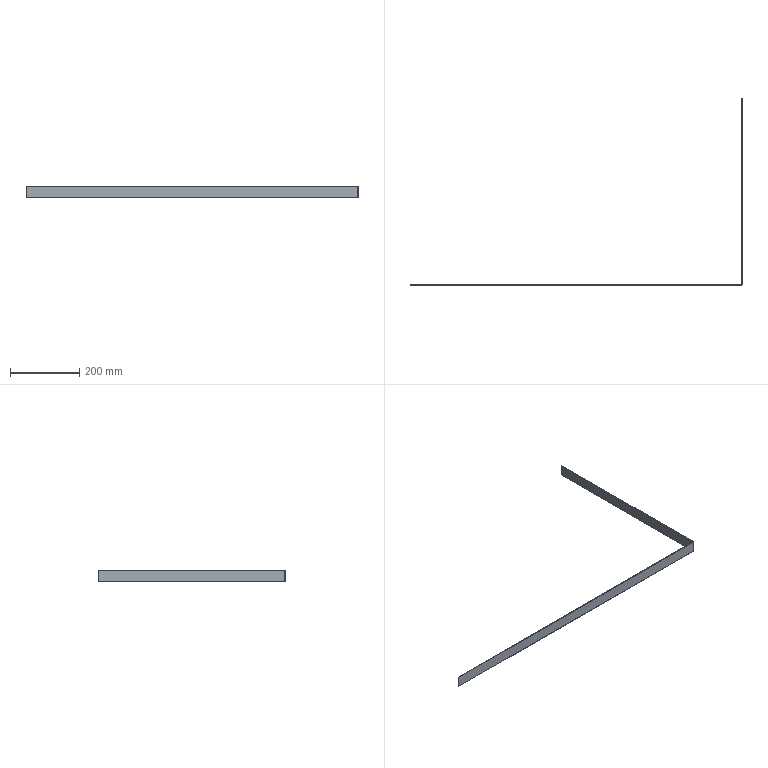Part | SolidWorks | features FlatPattern 1, SMBaseFlange 1, SheetMetal 1 | 1 solid | 14 faces | box 957.6 x 538.5 x 32 mm | volume 71721 mm3 | plane 12 | cylinder 2 | commonest cylinder face diameters 0.4 x1 3.4 x1
STEP:
#1=CARTESIAN_POINT('',(956.1,0.2,32.));
#2=VERTEX_POINT('',#1);
#3=CARTESIAN_POINT('',(957.6,0.2,32.));
#4=VERTEX_POINT('',#3);
#5=CARTESIAN_POINT('',(956.1,0.2,32.));
#6=DIRECTION('',(1.,0.,0.));
#7=VECTOR('',#6,1000.);
#8=LINE('',#5,#7);
#9=EDGE_CURVE('',#2,#4,#8,.T.);
#10=ORIENTED_EDGE('',*,*,#9,.F.);
#11=CARTESIAN_POINT('',(955.9,0.,32.));
#12=VERTEX_POINT('',#11);
#13=CARTESIAN_POINT('',(955.9,0.2,32.));
#14=DIRECTION('',(0.,0.,1.));
#15=DIRECTION('',(-1.,0.,0.));
#16=AXIS2_PLACEMENT_3D('',#13,#14,#15);
#17=CIRCLE('',#16,0.2);
#18=EDGE_CURVE('',#12,#2,#17,.T.);
#19=ORIENTED_EDGE('',*,*,#18,.F.);
#20=CARTESIAN_POINT('',(955.9,-1.5,32.));
#21=VERTEX_POINT('',#20);
#22=CARTESIAN_POINT('',(955.9,-1.5,32.));
#23=DIRECTION('',(0.,1.,0.));
#24=VECTOR('',#23,1000.);
#25=LINE('',#22,#24);
#26=EDGE_CURVE('',#21,#12,#25,.T.);
#27=ORIENTED_EDGE('',*,*,#26,.F.);
#28=CARTESIAN_POINT('',(955.9,0.2,32.));
#29=DIRECTION('',(0.,0.,1.));
#30=DIRECTION('',(1.,0.,0.));
#31=AXIS2_PLACEMENT_3D('',#28,#29,#30);
#32=CIRCLE('',#31,1.7);
#33=EDGE_CURVE('',#21,#4,#32,.T.);
#34=ORIENTED_EDGE('',*,*,#33,.T.);
#35=EDGE_LOOP('',(#10,#19,#27,#34));
#36=FACE_OUTER_BOUND('',#35,.T.);
#37=CARTESIAN_POINT('',(956.1,0.2,32.));
#38=DIRECTION('',(0.,0.,1.));
#39=DIRECTION('',(1.,0.,0.));
#40=AXIS2_PLACEMENT_3D('',#37,#38,#39);
#41=PLANE('',#40);
#42=ADVANCED_FACE('',(#36),#41,.T.);
#43=CARTESIAN_POINT('',(956.1,537.,32.));
#44=VERTEX_POINT('',#43);
#45=CARTESIAN_POINT('',(956.1,0.,32.));
#46=DIRECTION('',(0.,1.,0.));
#47=VECTOR('',#46,1000.);
#48=LINE('',#45,#47);
#49=EDGE_CURVE('',#2,#44,#48,.T.);
#50=ORIENTED_EDGE('',*,*,#49,.F.);
#51=ORIENTED_EDGE('',*,*,#9,.T.);
#52=CARTESIAN_POINT('',(957.6,537.,32.));
#53=VERTEX_POINT('',#52);
#54=CARTESIAN_POINT('',(957.6,0.,32.));
#55=DIRECTION('',(0.,1.,0.));
#56=VECTOR('',#55,1000.);
#57=LINE('',#54,#56);
#58=EDGE_CURVE('',#4,#53,#57,.T.);
#59=ORIENTED_EDGE('',*,*,#58,.T.);
#60=CARTESIAN_POINT('',(956.1,537.,32.));
#61=DIRECTION('',(1.,0.,0.));
#62=VECTOR('',#61,1000.);
#63=LINE('',#60,#62);
#64=EDGE_CURVE('',#44,#53,#63,.T.);
#65=ORIENTED_EDGE('',*,*,#64,.F.);
#66=EDGE_LOOP('',(#50,#51,#59,#65));
#67=FACE_OUTER_BOUND('',#66,.T.);
#68=CARTESIAN_POINT('',(955.9,-1.5,32.));
#69=DIRECTION('',(0.,0.,1.));
#70=DIRECTION('',(1.,0.,0.));
#71=AXIS2_PLACEMENT_3D('',#68,#69,#70);
#72=PLANE('',#71);
#73=ADVANCED_FACE('',(#67),#72,.T.);
#74=CARTESIAN_POINT('',(955.9,0.,0.));
#75=VERTEX_POINT('',#74);
#76=CARTESIAN_POINT('',(955.9,-1.5,0.));
#77=VERTEX_POINT('',#76);
#78=CARTESIAN_POINT('',(955.9,0.,0.));
#79=DIRECTION('',(0.,-1.,0.));
#80=VECTOR('',#79,1000.);
#81=LINE('',#78,#80);
#82=EDGE_CURVE('',#75,#77,#81,.T.);
#83=ORIENTED_EDGE('',*,*,#82,.F.);
#84=CARTESIAN_POINT('',(956.1,0.2,0.));
#85=VERTEX_POINT('',#84);
#86=CARTESIAN_POINT('',(955.9,0.2,0.));
#87=DIRECTION('',(0.,0.,1.));
#88=DIRECTION('',(-1.,0.,0.));
#89=AXIS2_PLACEMENT_3D('',#86,#87,#88);
#90=CIRCLE('',#89,0.2);
#91=EDGE_CURVE('',#75,#85,#90,.T.);
#92=ORIENTED_EDGE('',*,*,#91,.T.);
#93=CARTESIAN_POINT('',(957.6,0.2,0.));
#94=VERTEX_POINT('',#93);
#95=CARTESIAN_POINT('',(957.6,0.2,0.));
#96=DIRECTION('',(-1.,0.,0.));
#97=VECTOR('',#96,1000.);
#98=LINE('',#95,#97);
#99=EDGE_CURVE('',#94,#85,#98,.T.);
#100=ORIENTED_EDGE('',*,*,#99,.F.);
#101=CARTESIAN_POINT('',(955.9,0.2,0.));
#102=DIRECTION('',(0.,0.,1.));
#103=DIRECTION('',(1.,0.,0.));
#104=AXIS2_PLACEMENT_3D('',#101,#102,#103);
#105=CIRCLE('',#104,1.7);
#106=EDGE_CURVE('',#77,#94,#105,.T.);
#107=ORIENTED_EDGE('',*,*,#106,.F.);
#108=EDGE_LOOP('',(#83,#92,#100,#107));
#109=FACE_OUTER_BOUND('',#108,.T.);
#110=CARTESIAN_POINT('',(955.9,0.,0.));
#111=DIRECTION('',(0.,0.,-1.));
#112=DIRECTION('',(-1.,0.,0.));
#113=AXIS2_PLACEMENT_3D('',#110,#111,#112);
#114=PLANE('',#113);
#115=ADVANCED_FACE('',(#109),#114,.T.);
#116=CARTESIAN_POINT('',(0.,0.,0.));
#117=VERTEX_POINT('',#116);
#118=CARTESIAN_POINT('',(0.,0.,0.));
#119=DIRECTION('',(1.,0.,0.));
#120=VECTOR('',#119,1000.);
#121=LINE('',#118,#120);
#122=EDGE_CURVE('',#117,#75,#121,.T.);
#123=ORIENTED_EDGE('',*,*,#122,.T.);
#124=ORIENTED_EDGE('',*,*,#82,.T.);
#125=CARTESIAN_POINT('',(0.,-1.5,0.));
#126=VERTEX_POINT('',#125);
#127=CARTESIAN_POINT('',(0.,-1.5,0.));
#128=DIRECTION('',(1.,0.,0.));
#129=VECTOR('',#128,1000.);
#130=LINE('',#127,#129);
#131=EDGE_CURVE('',#126,#77,#130,.T.);
#132=ORIENTED_EDGE('',*,*,#131,.F.);
#133=CARTESIAN_POINT('',(0.,-1.5,0.));
#134=DIRECTION('',(0.,1.,0.));
#135=VECTOR('',#134,1000.);
#136=LINE('',#133,#135);
#137=EDGE_CURVE('',#126,#117,#136,.T.);
#138=ORIENTED_EDGE('',*,*,#137,.T.);
#139=EDGE_LOOP('',(#123,#124,#132,#138));
#140=FACE_OUTER_BOUND('',#139,.T.);
#141=CARTESIAN_POINT('',(957.6,0.2,0.));
#142=DIRECTION('',(0.,0.,-1.));
#143=DIRECTION('',(-1.,0.,0.));
#144=AXIS2_PLACEMENT_3D('',#141,#142,#143);
#145=PLANE('',#144);
#146=ADVANCED_FACE('',(#140),#145,.T.);
#147=CARTESIAN_POINT('',(957.6,537.,0.));
#148=VERTEX_POINT('',#147);
#149=CARTESIAN_POINT('',(957.6,0.,0.));
#150=DIRECTION('',(0.,1.,0.));
#151=VECTOR('',#150,1000.);
#152=LINE('',#149,#151);
#153=EDGE_CURVE('',#94,#148,#152,.T.);
#154=ORIENTED_EDGE('',*,*,#153,.T.);
#155=CARTESIAN_POINT('',(957.6,537.,32.));
#156=DIRECTION('',(0.,0.,-1.));
#157=VECTOR('',#156,1000.);
#158=LINE('',#155,#157);
#159=EDGE_CURVE('',#53,#148,#158,.T.);
#160=ORIENTED_EDGE('',*,*,#159,.F.);
#161=ORIENTED_EDGE('',*,*,#58,.F.);
#162=CARTESIAN_POINT('',(957.6,0.2,32.));
#163=DIRECTION('',(0.,0.,-1.));
#164=VECTOR('',#163,1000.);
#165=LINE('',#162,#164);
#166=EDGE_CURVE('',#4,#94,#165,.T.);
#167=ORIENTED_EDGE('',*,*,#166,.T.);
#168=EDGE_LOOP('',(#154,#160,#161,#167));
#169=FACE_OUTER_BOUND('',#168,.T.);
#170=CARTESIAN_POINT('',(957.6,0.,32.));
#171=DIRECTION('',(-1.,0.,0.));
#172=DIRECTION('',(0.,0.,1.));
#173=AXIS2_PLACEMENT_3D('',#170,#171,#172);
#174=PLANE('',#173);
#175=ADVANCED_FACE('',(#169),#174,.F.);
#176=CARTESIAN_POINT('',(956.1,537.,0.));
#177=VERTEX_POINT('',#176);
#178=CARTESIAN_POINT('',(956.1,537.,0.));
#179=DIRECTION('',(1.,0.,0.));
#180=VECTOR('',#179,1000.);
#181=LINE('',#178,#180);
#182=EDGE_CURVE('',#177,#148,#181,.T.);
#183=ORIENTED_EDGE('',*,*,#182,.F.);
#184=CARTESIAN_POINT('',(956.1,537.,32.));
#185=DIRECTION('',(0.,0.,-1.));
#186=VECTOR('',#185,1000.);
#187=LINE('',#184,#186);
#188=EDGE_CURVE('',#44,#177,#187,.T.);
#189=ORIENTED_EDGE('',*,*,#188,.F.);
#190=ORIENTED_EDGE('',*,*,#64,.T.);
#191=ORIENTED_EDGE('',*,*,#159,.T.);
#192=EDGE_LOOP('',(#183,#189,#190,#191));
#193=FACE_OUTER_BOUND('',#192,.T.);
#194=CARTESIAN_POINT('',(956.1,537.,32.));
#195=DIRECTION('',(0.,1.,0.));
#196=DIRECTION('',(0.,0.,1.));
#197=AXIS2_PLACEMENT_3D('',#194,#195,#196);
#198=PLANE('',#197);
#199=ADVANCED_FACE('',(#193),#198,.T.);
#200=CARTESIAN_POINT('',(956.1,0.,0.));
#201=DIRECTION('',(0.,1.,0.));
#202=VECTOR('',#201,1000.);
#203=LINE('',#200,#202);
#204=EDGE_CURVE('',#85,#177,#203,.T.);
#205=ORIENTED_EDGE('',*,*,#204,.F.);
#206=CARTESIAN_POINT('',(956.1,0.2,32.));
#207=DIRECTION('',(0.,0.,-1.));
#208=VECTOR('',#207,1000.);
#209=LINE('',#206,#208);
#210=EDGE_CURVE('',#2,#85,#209,.T.);
#211=ORIENTED_EDGE('',*,*,#210,.F.);
#212=ORIENTED_EDGE('',*,*,#49,.T.);
#213=ORIENTED_EDGE('',*,*,#188,.T.);
#214=EDGE_LOOP('',(#205,#211,#212,#213));
#215=FACE_OUTER_BOUND('',#214,.T.);
#216=CARTESIAN_POINT('',(956.1,0.,32.));
#217=DIRECTION('',(-1.,0.,0.));
#218=DIRECTION('',(0.,0.,1.));
#219=AXIS2_PLACEMENT_3D('',#216,#217,#218);
#220=PLANE('',#219);
#221=ADVANCED_FACE('',(#215),#220,.T.);
#222=ORIENTED_EDGE('',*,*,#91,.F.);
#223=CARTESIAN_POINT('',(955.9,0.,32.));
#224=DIRECTION('',(0.,0.,-1.));
#225=VECTOR('',#224,1000.);
#226=LINE('',#223,#225);
#227=EDGE_CURVE('',#12,#75,#226,.T.);
#228=ORIENTED_EDGE('',*,*,#227,.F.);
#229=ORIENTED_EDGE('',*,*,#18,.T.);
#230=ORIENTED_EDGE('',*,*,#210,.T.);
#231=EDGE_LOOP('',(#222,#228,#229,#230));
#232=FACE_OUTER_BOUND('',#231,.T.);
#233=CARTESIAN_POINT('',(955.9,0.2,32.));
#234=DIRECTION('',(0.,0.,-1.));
#235=DIRECTION('',(-1.,0.,0.));
#236=AXIS2_PLACEMENT_3D('',#233,#234,#235);
#237=CYLINDRICAL_SURFACE('',#236,0.2);
#238=ADVANCED_FACE('',(#232),#237,.F.);
#239=ORIENTED_EDGE('',*,*,#122,.F.);
#240=CARTESIAN_POINT('',(0.,0.,32.));
#241=VERTEX_POINT('',#240);
#242=CARTESIAN_POINT('',(0.,0.,32.));
#243=DIRECTION('',(0.,0.,-1.));
#244=VECTOR('',#243,1000.);
#245=LINE('',#242,#244);
#246=EDGE_CURVE('',#241,#117,#245,.T.);
#247=ORIENTED_EDGE('',*,*,#246,.F.);
#248=CARTESIAN_POINT('',(0.,0.,32.));
#249=DIRECTION('',(1.,0.,0.));
#250=VECTOR('',#249,1000.);
#251=LINE('',#248,#250);
#252=EDGE_CURVE('',#241,#12,#251,.T.);
#253=ORIENTED_EDGE('',*,*,#252,.T.);
#254=ORIENTED_EDGE('',*,*,#227,.T.);
#255=EDGE_LOOP('',(#239,#247,#253,#254));
#256=FACE_OUTER_BOUND('',#255,.T.);
#257=CARTESIAN_POINT('',(0.,0.,32.));
#258=DIRECTION('',(0.,1.,0.));
#259=DIRECTION('',(0.,0.,1.));
#260=AXIS2_PLACEMENT_3D('',#257,#258,#259);
#261=PLANE('',#260);
#262=ADVANCED_FACE('',(#256),#261,.T.);
#263=ORIENTED_EDGE('',*,*,#137,.F.);
#264=CARTESIAN_POINT('',(0.,-1.5,32.));
#265=VERTEX_POINT('',#264);
#266=CARTESIAN_POINT('',(0.,-1.5,32.));
#267=DIRECTION('',(0.,0.,-1.));
#268=VECTOR('',#267,1000.);
#269=LINE('',#266,#268);
#270=EDGE_CURVE('',#265,#126,#269,.T.);
#271=ORIENTED_EDGE('',*,*,#270,.F.);
#272=CARTESIAN_POINT('',(0.,-1.5,32.));
#273=DIRECTION('',(0.,1.,0.));
#274=VECTOR('',#273,1000.);
#275=LINE('',#272,#274);
#276=EDGE_CURVE('',#265,#241,#275,.T.);
#277=ORIENTED_EDGE('',*,*,#276,.T.);
#278=ORIENTED_EDGE('',*,*,#246,.T.);
#279=EDGE_LOOP('',(#263,#271,#277,#278));
#280=FACE_OUTER_BOUND('',#279,.T.);
#281=CARTESIAN_POINT('',(0.,-1.5,32.));
#282=DIRECTION('',(-1.,0.,0.));
#283=DIRECTION('',(0.,0.,1.));
#284=AXIS2_PLACEMENT_3D('',#281,#282,#283);
#285=PLANE('',#284);
#286=ADVANCED_FACE('',(#280),#285,.T.);
#287=ORIENTED_EDGE('',*,*,#131,.T.);
#288=CARTESIAN_POINT('',(955.9,-1.5,32.));
#289=DIRECTION('',(0.,0.,-1.));
#290=VECTOR('',#289,1000.);
#291=LINE('',#288,#290);
#292=EDGE_CURVE('',#21,#77,#291,.T.);
#293=ORIENTED_EDGE('',*,*,#292,.F.);
#294=CARTESIAN_POINT('',(0.,-1.5,32.));
#295=DIRECTION('',(1.,0.,0.));
#296=VECTOR('',#295,1000.);
#297=LINE('',#294,#296);
#298=EDGE_CURVE('',#265,#21,#297,.T.);
#299=ORIENTED_EDGE('',*,*,#298,.F.);
#300=ORIENTED_EDGE('',*,*,#270,.T.);
#301=EDGE_LOOP('',(#287,#293,#299,#300));
#302=FACE_OUTER_BOUND('',#301,.T.);
#303=CARTESIAN_POINT('',(0.,-1.5,32.));
#304=DIRECTION('',(0.,1.,0.));
#305=DIRECTION('',(0.,0.,1.));
#306=AXIS2_PLACEMENT_3D('',#303,#304,#305);
#307=PLANE('',#306);
#308=ADVANCED_FACE('',(#302),#307,.F.);
#309=ORIENTED_EDGE('',*,*,#106,.T.);
#310=ORIENTED_EDGE('',*,*,#166,.F.);
#311=ORIENTED_EDGE('',*,*,#33,.F.);
#312=ORIENTED_EDGE('',*,*,#292,.T.);
#313=EDGE_LOOP('',(#309,#310,#311,#312));
#314=FACE_OUTER_BOUND('',#313,.T.);
#315=CARTESIAN_POINT('',(955.9,0.2,32.));
#316=DIRECTION('',(0.,0.,-1.));
#317=DIRECTION('',(-1.,0.,0.));
#318=AXIS2_PLACEMENT_3D('',#315,#316,#317);
#319=CYLINDRICAL_SURFACE('',#318,1.7);
#320=ADVANCED_FACE('',(#314),#319,.T.);
#321=ORIENTED_EDGE('',*,*,#298,.T.);
#322=ORIENTED_EDGE('',*,*,#26,.T.);
#323=ORIENTED_EDGE('',*,*,#252,.F.);
#324=ORIENTED_EDGE('',*,*,#276,.F.);
#325=EDGE_LOOP('',(#321,#322,#323,#324));
#326=FACE_OUTER_BOUND('',#325,.T.);
#327=CARTESIAN_POINT('',(955.9,0.2,32.));
#328=DIRECTION('',(0.,0.,-1.));
#329=DIRECTION('',(-1.,0.,0.));
#330=AXIS2_PLACEMENT_3D('',#327,#328,#329);
#331=PLANE('',#330);
#332=ADVANCED_FACE('',(#326),#331,.F.);
#333=ORIENTED_EDGE('',*,*,#153,.F.);
#334=ORIENTED_EDGE('',*,*,#99,.T.);
#335=ORIENTED_EDGE('',*,*,#204,.T.);
#336=ORIENTED_EDGE('',*,*,#182,.T.);
#337=EDGE_LOOP('',(#333,#334,#335,#336));
#338=FACE_OUTER_BOUND('',#337,.T.);
#339=CARTESIAN_POINT('',(955.9,0.2,0.));
#340=DIRECTION('',(0.,0.,-1.));
#341=DIRECTION('',(-1.,0.,0.));
#342=AXIS2_PLACEMENT_3D('',#339,#340,#341);
#343=PLANE('',#342);
#344=ADVANCED_FACE('',(#338),#343,.T.);
#345=CLOSED_SHELL('',(#42,#73,#115,#146,#175,#199,#221,#238,#262,#286,#308,#320,#332,#344));
#346=MANIFOLD_SOLID_BREP('',#345);
#347=CARTESIAN_POINT('',(0.,0.,0.));
#348=DIRECTION('',(0.,0.,1.));
#349=DIRECTION('',(1.,0.,0.));
#350=AXIS2_PLACEMENT_3D('',#347,#348,#349);
#351=(LENGTH_UNIT()NAMED_UNIT(*)SI_UNIT(.MILLI.,.METRE.));
#352=UNCERTAINTY_MEASURE_WITH_UNIT(LENGTH_MEASURE(0.00001),#351,'','');
#353=(NAMED_UNIT(*)PLANE_ANGLE_UNIT()SI_UNIT($,.RADIAN.));
#354=(NAMED_UNIT(*)SI_UNIT($,.STERADIAN.)SOLID_ANGLE_UNIT());
#355=(GEOMETRIC_REPRESENTATION_CONTEXT(3)GLOBAL_UNCERTAINTY_ASSIGNED_CONTEXT((#352))GLOBAL_UNIT_ASSIGNED_CONTEXT((#351,#353,#354))REPRESENTATION_CONTEXT('',''));
#356=ADVANCED_BREP_SHAPE_REPRESENTATION('',(#346,#350),#355);